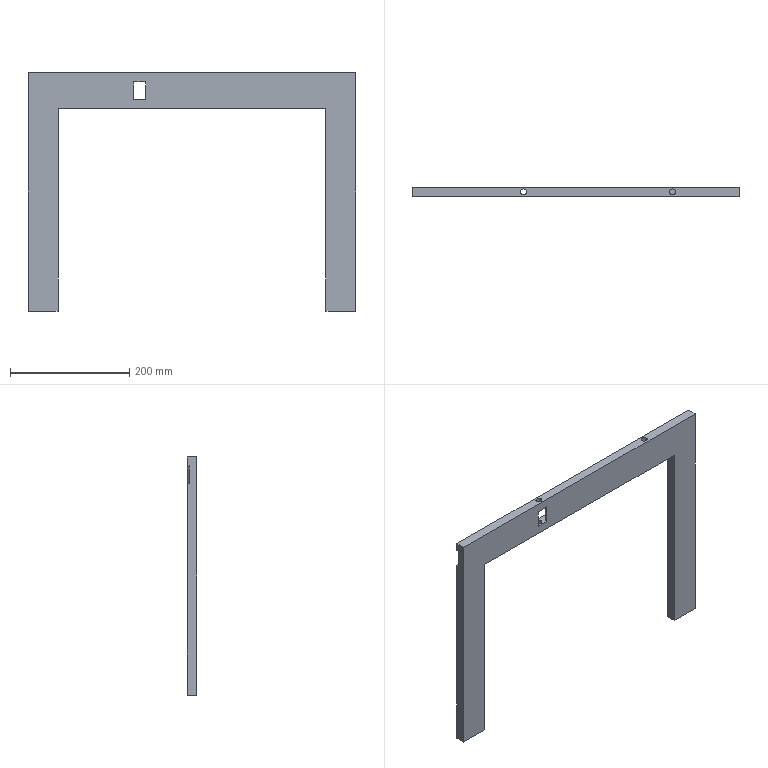Part | SolidWorks | features ICE 10, HoleWzd 3, Extrusion 1 | 1 solid | 25 faces | box 550 x 16 x 400 mm | volume 983083 mm3 | plane 19 | cylinder 6 | commonest cylinder face diameters 10 x6
STEP:
#1=CARTESIAN_POINT('',(182.,-8.,-60.));
#2=VERTEX_POINT('',#1);
#3=CARTESIAN_POINT('',(192.,-8.,-60.));
#4=VERTEX_POINT('',#3);
#5=CARTESIAN_POINT('',(187.,-8.,-60.));
#6=DIRECTION('',(0.,0.,1.));
#7=DIRECTION('',(1.,0.,0.));
#8=AXIS2_PLACEMENT_3D('',#5,#6,#7);
#9=CIRCLE('',#8,5.);
#10=EDGE_CURVE('',#2,#4,#9,.T.);
#11=ORIENTED_EDGE('',*,*,#10,.F.);
#12=CARTESIAN_POINT('',(182.,-8.,-45.));
#13=VERTEX_POINT('',#12);
#14=CARTESIAN_POINT('',(182.,-8.,-45.));
#15=DIRECTION('',(0.,0.,1.));
#16=VECTOR('',#15,1000.);
#17=LINE('',#14,#16);
#18=EDGE_CURVE('',#2,#13,#17,.T.);
#19=ORIENTED_EDGE('',*,*,#18,.T.);
#20=CARTESIAN_POINT('',(192.,-8.,-45.));
#21=VERTEX_POINT('',#20);
#22=CARTESIAN_POINT('',(187.,-8.,-45.));
#23=DIRECTION('',(0.,0.,1.));
#24=DIRECTION('',(1.,0.,0.));
#25=AXIS2_PLACEMENT_3D('',#22,#23,#24);
#26=CIRCLE('',#25,5.);
#27=EDGE_CURVE('',#13,#21,#26,.T.);
#28=ORIENTED_EDGE('',*,*,#27,.T.);
#29=CARTESIAN_POINT('',(192.,-8.,-45.));
#30=DIRECTION('',(0.,0.,1.));
#31=VECTOR('',#30,1000.);
#32=LINE('',#29,#31);
#33=EDGE_CURVE('',#4,#21,#32,.T.);
#34=ORIENTED_EDGE('',*,*,#33,.F.);
#35=EDGE_LOOP('',(#11,#19,#28,#34));
#36=FACE_OUTER_BOUND('',#35,.T.);
#37=CARTESIAN_POINT('',(187.,-8.,-45.));
#38=DIRECTION('',(0.,0.,1.));
#39=DIRECTION('',(1.,0.,0.));
#40=AXIS2_PLACEMENT_3D('',#37,#38,#39);
#41=CYLINDRICAL_SURFACE('',#40,5.);
#42=ADVANCED_FACE('',(#36),#41,.F.);
#43=CARTESIAN_POINT('',(192.,-8.,-15.));
#44=VERTEX_POINT('',#43);
#45=CARTESIAN_POINT('',(182.,-8.,-15.));
#46=VERTEX_POINT('',#45);
#47=CARTESIAN_POINT('',(187.,-8.,-15.));
#48=DIRECTION('',(0.,0.,-1.));
#49=DIRECTION('',(-1.,0.,0.));
#50=AXIS2_PLACEMENT_3D('',#47,#48,#49);
#51=CIRCLE('',#50,5.);
#52=EDGE_CURVE('',#44,#46,#51,.T.);
#53=ORIENTED_EDGE('',*,*,#52,.T.);
#54=CARTESIAN_POINT('',(182.,-8.,0.));
#55=VERTEX_POINT('',#54);
#56=CARTESIAN_POINT('',(182.,-8.,0.));
#57=DIRECTION('',(0.,0.,1.));
#58=VECTOR('',#57,1000.);
#59=LINE('',#56,#58);
#60=EDGE_CURVE('',#46,#55,#59,.T.);
#61=ORIENTED_EDGE('',*,*,#60,.T.);
#62=CARTESIAN_POINT('',(192.,-8.,0.));
#63=VERTEX_POINT('',#62);
#64=CARTESIAN_POINT('',(187.,-8.,0.));
#65=DIRECTION('',(0.,0.,1.));
#66=DIRECTION('',(1.,0.,0.));
#67=AXIS2_PLACEMENT_3D('',#64,#65,#66);
#68=CIRCLE('',#67,5.);
#69=EDGE_CURVE('',#55,#63,#68,.T.);
#70=ORIENTED_EDGE('',*,*,#69,.T.);
#71=CARTESIAN_POINT('',(192.,-8.,0.));
#72=DIRECTION('',(0.,0.,1.));
#73=VECTOR('',#72,1000.);
#74=LINE('',#71,#73);
#75=EDGE_CURVE('',#44,#63,#74,.T.);
#76=ORIENTED_EDGE('',*,*,#75,.F.);
#77=EDGE_LOOP('',(#53,#61,#70,#76));
#78=FACE_OUTER_BOUND('',#77,.T.);
#79=CARTESIAN_POINT('',(187.,-8.,0.));
#80=DIRECTION('',(0.,0.,1.));
#81=DIRECTION('',(1.,0.,0.));
#82=AXIS2_PLACEMENT_3D('',#79,#80,#81);
#83=CYLINDRICAL_SURFACE('',#82,5.);
#84=ADVANCED_FACE('',(#78),#83,.F.);
#85=CARTESIAN_POINT('',(432.,-8.,-20.));
#86=VERTEX_POINT('',#85);
#87=CARTESIAN_POINT('',(442.,-8.,-20.));
#88=VERTEX_POINT('',#87);
#89=CARTESIAN_POINT('',(437.,-8.,-20.));
#90=DIRECTION('',(0.,0.,1.));
#91=DIRECTION('',(1.,0.,0.));
#92=AXIS2_PLACEMENT_3D('',#89,#90,#91);
#93=CIRCLE('',#92,5.);
#94=EDGE_CURVE('',#86,#88,#93,.T.);
#95=ORIENTED_EDGE('',*,*,#94,.F.);
#96=CARTESIAN_POINT('',(432.,-8.,0.));
#97=VERTEX_POINT('',#96);
#98=CARTESIAN_POINT('',(432.,-8.,0.));
#99=DIRECTION('',(0.,0.,1.));
#100=VECTOR('',#99,1000.);
#101=LINE('',#98,#100);
#102=EDGE_CURVE('',#86,#97,#101,.T.);
#103=ORIENTED_EDGE('',*,*,#102,.T.);
#104=CARTESIAN_POINT('',(442.,-8.,0.));
#105=VERTEX_POINT('',#104);
#106=CARTESIAN_POINT('',(437.,-8.,0.));
#107=DIRECTION('',(0.,0.,1.));
#108=DIRECTION('',(1.,0.,0.));
#109=AXIS2_PLACEMENT_3D('',#106,#107,#108);
#110=CIRCLE('',#109,5.);
#111=EDGE_CURVE('',#97,#105,#110,.T.);
#112=ORIENTED_EDGE('',*,*,#111,.T.);
#113=CARTESIAN_POINT('',(442.,-8.,0.));
#114=DIRECTION('',(0.,0.,1.));
#115=VECTOR('',#114,1000.);
#116=LINE('',#113,#115);
#117=EDGE_CURVE('',#88,#105,#116,.T.);
#118=ORIENTED_EDGE('',*,*,#117,.F.);
#119=EDGE_LOOP('',(#95,#103,#112,#118));
#120=FACE_OUTER_BOUND('',#119,.T.);
#121=CARTESIAN_POINT('',(437.,-8.,0.));
#122=DIRECTION('',(0.,0.,1.));
#123=DIRECTION('',(1.,0.,0.));
#124=AXIS2_PLACEMENT_3D('',#121,#122,#123);
#125=CYLINDRICAL_SURFACE('',#124,5.);
#126=ADVANCED_FACE('',(#120),#125,.F.);
#127=CARTESIAN_POINT('',(437.,-8.,0.));
#128=DIRECTION('',(0.,0.,1.));
#129=DIRECTION('',(1.,0.,0.));
#130=AXIS2_PLACEMENT_3D('',#127,#128,#129);
#131=CIRCLE('',#130,5.);
#132=EDGE_CURVE('',#105,#97,#131,.T.);
#133=ORIENTED_EDGE('',*,*,#132,.F.);
#134=ORIENTED_EDGE('',*,*,#111,.F.);
#135=EDGE_LOOP('',(#133,#134));
#136=FACE_BOUND('',#135,.T.);
#137=CARTESIAN_POINT('',(0.,-16.,0.));
#138=VERTEX_POINT('',#137);
#139=CARTESIAN_POINT('',(550.,-16.,0.));
#140=VERTEX_POINT('',#139);
#141=CARTESIAN_POINT('',(355.,-16.,0.));
#142=DIRECTION('',(1.,0.,0.));
#143=VECTOR('',#142,1000.);
#144=LINE('',#141,#143);
#145=EDGE_CURVE('',#138,#140,#144,.T.);
#146=ORIENTED_EDGE('',*,*,#145,.T.);
#147=CARTESIAN_POINT('',(550.,0.,0.));
#148=VERTEX_POINT('',#147);
#149=CARTESIAN_POINT('',(550.,-16.,0.));
#150=DIRECTION('',(0.,-1.,0.));
#151=VECTOR('',#150,1000.);
#152=LINE('',#149,#151);
#153=EDGE_CURVE('',#148,#140,#152,.T.);
#154=ORIENTED_EDGE('',*,*,#153,.F.);
#155=CARTESIAN_POINT('',(0.,0.,0.));
#156=VERTEX_POINT('',#155);
#157=CARTESIAN_POINT('',(347.,0.,0.));
#158=DIRECTION('',(-1.,0.,0.));
#159=VECTOR('',#158,1000.);
#160=LINE('',#157,#159);
#161=EDGE_CURVE('',#148,#156,#160,.T.);
#162=ORIENTED_EDGE('',*,*,#161,.T.);
#163=CARTESIAN_POINT('',(0.,0.,0.));
#164=DIRECTION('',(0.,1.,0.));
#165=VECTOR('',#164,1000.);
#166=LINE('',#163,#165);
#167=EDGE_CURVE('',#138,#156,#166,.T.);
#168=ORIENTED_EDGE('',*,*,#167,.F.);
#169=EDGE_LOOP('',(#146,#154,#162,#168));
#170=FACE_OUTER_BOUND('',#169,.T.);
#171=CARTESIAN_POINT('',(187.,-8.,0.));
#172=DIRECTION('',(0.,0.,1.));
#173=DIRECTION('',(1.,0.,0.));
#174=AXIS2_PLACEMENT_3D('',#171,#172,#173);
#175=CIRCLE('',#174,5.);
#176=EDGE_CURVE('',#63,#55,#175,.T.);
#177=ORIENTED_EDGE('',*,*,#176,.F.);
#178=ORIENTED_EDGE('',*,*,#69,.F.);
#179=EDGE_LOOP('',(#177,#178));
#180=FACE_BOUND('',#179,.T.);
#181=CARTESIAN_POINT('',(0.,0.,0.));
#182=DIRECTION('',(0.,0.,-1.));
#183=DIRECTION('',(-1.,0.,0.));
#184=AXIS2_PLACEMENT_3D('',#181,#182,#183);
#185=PLANE('',#184);
#186=ADVANCED_FACE('',(#136,#170,#180),#185,.F.);
#187=CARTESIAN_POINT('',(550.,-16.,-400.));
#188=VERTEX_POINT('',#187);
#189=CARTESIAN_POINT('',(500.,-16.,-400.));
#190=VERTEX_POINT('',#189);
#191=CARTESIAN_POINT('',(0.,-16.,-400.));
#192=DIRECTION('',(-1.,0.,0.));
#193=VECTOR('',#192,1000.);
#194=LINE('',#191,#193);
#195=EDGE_CURVE('',#188,#190,#194,.T.);
#196=ORIENTED_EDGE('',*,*,#195,.T.);
#197=CARTESIAN_POINT('',(500.,0.,-400.));
#198=VERTEX_POINT('',#197);
#199=CARTESIAN_POINT('',(500.,-16.,-400.));
#200=DIRECTION('',(0.,1.,0.));
#201=VECTOR('',#200,1000.);
#202=LINE('',#199,#201);
#203=EDGE_CURVE('',#190,#198,#202,.T.);
#204=ORIENTED_EDGE('',*,*,#203,.T.);
#205=CARTESIAN_POINT('',(550.,0.,-400.));
#206=VERTEX_POINT('',#205);
#207=CARTESIAN_POINT('',(550.,0.,-400.));
#208=DIRECTION('',(1.,0.,0.));
#209=VECTOR('',#208,1000.);
#210=LINE('',#207,#209);
#211=EDGE_CURVE('',#198,#206,#210,.T.);
#212=ORIENTED_EDGE('',*,*,#211,.T.);
#213=CARTESIAN_POINT('',(550.,-16.,-400.));
#214=DIRECTION('',(0.,-1.,0.));
#215=VECTOR('',#214,1000.);
#216=LINE('',#213,#215);
#217=EDGE_CURVE('',#206,#188,#216,.T.);
#218=ORIENTED_EDGE('',*,*,#217,.T.);
#219=EDGE_LOOP('',(#196,#204,#212,#218));
#220=FACE_OUTER_BOUND('',#219,.T.);
#221=CARTESIAN_POINT('',(0.,0.,-400.));
#222=DIRECTION('',(0.,0.,1.));
#223=DIRECTION('',(1.,0.,0.));
#224=AXIS2_PLACEMENT_3D('',#221,#222,#223);
#225=PLANE('',#224);
#226=ADVANCED_FACE('',(#220),#225,.F.);
#227=CARTESIAN_POINT('',(197.,-13.,-45.));
#228=VERTEX_POINT('',#227);
#229=CARTESIAN_POINT('',(197.,-13.,-15.));
#230=VERTEX_POINT('',#229);
#231=CARTESIAN_POINT('',(197.,-13.,-45.));
#232=DIRECTION('',(0.,0.,1.));
#233=VECTOR('',#232,1000.);
#234=LINE('',#231,#233);
#235=EDGE_CURVE('',#228,#230,#234,.T.);
#236=ORIENTED_EDGE('',*,*,#235,.F.);
#237=CARTESIAN_POINT('',(197.,-16.,-45.));
#238=VERTEX_POINT('',#237);
#239=CARTESIAN_POINT('',(197.,-16.,-45.));
#240=DIRECTION('',(0.,1.,0.));
#241=VECTOR('',#240,1000.);
#242=LINE('',#239,#241);
#243=EDGE_CURVE('',#238,#228,#242,.T.);
#244=ORIENTED_EDGE('',*,*,#243,.F.);
#245=CARTESIAN_POINT('',(197.,-16.,-15.));
#246=VERTEX_POINT('',#245);
#247=CARTESIAN_POINT('',(197.,-16.,-15.));
#248=DIRECTION('',(0.,0.,-1.));
#249=VECTOR('',#248,1000.);
#250=LINE('',#247,#249);
#251=EDGE_CURVE('',#246,#238,#250,.T.);
#252=ORIENTED_EDGE('',*,*,#251,.F.);
#253=CARTESIAN_POINT('',(197.,-3.,-15.));
#254=DIRECTION('',(0.,-1.,0.));
#255=VECTOR('',#254,1000.);
#256=LINE('',#253,#255);
#257=EDGE_CURVE('',#230,#246,#256,.T.);
#258=ORIENTED_EDGE('',*,*,#257,.F.);
#259=EDGE_LOOP('',(#236,#244,#252,#258));
#260=FACE_OUTER_BOUND('',#259,.T.);
#261=CARTESIAN_POINT('',(197.,0.,0.));
#262=DIRECTION('',(1.,0.,0.));
#263=DIRECTION('',(0.,0.,-1.));
#264=AXIS2_PLACEMENT_3D('',#261,#262,#263);
#265=PLANE('',#264);
#266=ADVANCED_FACE('',(#260),#265,.F.);
#267=CARTESIAN_POINT('',(0.,-3.,-15.));
#268=VERTEX_POINT('',#267);
#269=CARTESIAN_POINT('',(177.,-3.,-15.));
#270=VERTEX_POINT('',#269);
#271=CARTESIAN_POINT('',(0.,-3.,-15.));
#272=DIRECTION('',(1.,0.,0.));
#273=VECTOR('',#272,1000.);
#274=LINE('',#271,#273);
#275=EDGE_CURVE('',#268,#270,#274,.T.);
#276=ORIENTED_EDGE('',*,*,#275,.T.);
#277=CARTESIAN_POINT('',(177.,-3.,-45.));
#278=VERTEX_POINT('',#277);
#279=CARTESIAN_POINT('',(177.,-3.,-45.));
#280=DIRECTION('',(0.,0.,1.));
#281=VECTOR('',#280,1000.);
#282=LINE('',#279,#281);
#283=EDGE_CURVE('',#278,#270,#282,.T.);
#284=ORIENTED_EDGE('',*,*,#283,.F.);
#285=CARTESIAN_POINT('',(0.,-3.,-45.));
#286=VERTEX_POINT('',#285);
#287=CARTESIAN_POINT('',(347.,-3.,-45.));
#288=DIRECTION('',(-1.,0.,0.));
#289=VECTOR('',#288,1000.);
#290=LINE('',#287,#289);
#291=EDGE_CURVE('',#278,#286,#290,.T.);
#292=ORIENTED_EDGE('',*,*,#291,.T.);
#293=CARTESIAN_POINT('',(0.,-3.,-45.));
#294=DIRECTION('',(0.,0.,1.));
#295=VECTOR('',#294,1000.);
#296=LINE('',#293,#295);
#297=EDGE_CURVE('',#286,#268,#296,.T.);
#298=ORIENTED_EDGE('',*,*,#297,.T.);
#299=EDGE_LOOP('',(#276,#284,#292,#298));
#300=FACE_OUTER_BOUND('',#299,.T.);
#301=CARTESIAN_POINT('',(0.,-3.,0.));
#302=DIRECTION('',(0.,1.,0.));
#303=DIRECTION('',(0.,0.,1.));
#304=AXIS2_PLACEMENT_3D('',#301,#302,#303);
#305=PLANE('',#304);
#306=ADVANCED_FACE('',(#300),#305,.T.);
#307=CARTESIAN_POINT('',(177.,-16.,-45.));
#308=VERTEX_POINT('',#307);
#309=CARTESIAN_POINT('',(0.,-16.,-45.));
#310=DIRECTION('',(-1.,0.,0.));
#311=VECTOR('',#310,1000.);
#312=LINE('',#309,#311);
#313=EDGE_CURVE('',#238,#308,#312,.T.);
#314=ORIENTED_EDGE('',*,*,#313,.T.);
#315=CARTESIAN_POINT('',(177.,-16.,-15.));
#316=VERTEX_POINT('',#315);
#317=CARTESIAN_POINT('',(177.,-16.,-15.));
#318=DIRECTION('',(0.,0.,-1.));
#319=VECTOR('',#318,1000.);
#320=LINE('',#317,#319);
#321=EDGE_CURVE('',#316,#308,#320,.T.);
#322=ORIENTED_EDGE('',*,*,#321,.F.);
#323=CARTESIAN_POINT('',(177.,-16.,-15.));
#324=DIRECTION('',(1.,0.,0.));
#325=VECTOR('',#324,1000.);
#326=LINE('',#323,#325);
#327=EDGE_CURVE('',#316,#246,#326,.T.);
#328=ORIENTED_EDGE('',*,*,#327,.T.);
#329=ORIENTED_EDGE('',*,*,#251,.T.);
#330=EDGE_LOOP('',(#314,#322,#328,#329));
#331=FACE_BOUND('',#330,.T.);
#332=CARTESIAN_POINT('',(50.,-16.,-60.));
#333=VERTEX_POINT('',#332);
#334=CARTESIAN_POINT('',(500.,-16.,-60.));
#335=VERTEX_POINT('',#334);
#336=CARTESIAN_POINT('',(50.,-16.,-60.));
#337=DIRECTION('',(1.,0.,0.));
#338=VECTOR('',#337,1000.);
#339=LINE('',#336,#338);
#340=EDGE_CURVE('',#333,#335,#339,.T.);
#341=ORIENTED_EDGE('',*,*,#340,.T.);
#342=CARTESIAN_POINT('',(500.,-16.,-60.));
#343=DIRECTION('',(0.,0.,-1.));
#344=VECTOR('',#343,1000.);
#345=LINE('',#342,#344);
#346=EDGE_CURVE('',#335,#190,#345,.T.);
#347=ORIENTED_EDGE('',*,*,#346,.T.);
#348=ORIENTED_EDGE('',*,*,#195,.F.);
#349=CARTESIAN_POINT('',(550.,-16.,-45.));
#350=DIRECTION('',(0.,0.,-1.));
#351=VECTOR('',#350,1000.);
#352=LINE('',#349,#351);
#353=EDGE_CURVE('',#140,#188,#352,.T.);
#354=ORIENTED_EDGE('',*,*,#353,.F.);
#355=ORIENTED_EDGE('',*,*,#145,.F.);
#356=CARTESIAN_POINT('',(0.,-16.,-400.));
#357=VERTEX_POINT('',#356);
#358=CARTESIAN_POINT('',(0.,-16.,0.));
#359=DIRECTION('',(0.,0.,1.));
#360=VECTOR('',#359,1000.);
#361=LINE('',#358,#360);
#362=EDGE_CURVE('',#357,#138,#361,.T.);
#363=ORIENTED_EDGE('',*,*,#362,.F.);
#364=CARTESIAN_POINT('',(50.,-16.,-400.));
#365=VERTEX_POINT('',#364);
#366=CARTESIAN_POINT('',(0.,-16.,-400.));
#367=DIRECTION('',(-1.,0.,0.));
#368=VECTOR('',#367,1000.);
#369=LINE('',#366,#368);
#370=EDGE_CURVE('',#365,#357,#369,.T.);
#371=ORIENTED_EDGE('',*,*,#370,.F.);
#372=CARTESIAN_POINT('',(50.,-16.,-400.));
#373=DIRECTION('',(0.,0.,1.));
#374=VECTOR('',#373,1000.);
#375=LINE('',#372,#374);
#376=EDGE_CURVE('',#365,#333,#375,.T.);
#377=ORIENTED_EDGE('',*,*,#376,.T.);
#378=EDGE_LOOP('',(#341,#347,#348,#354,#355,#363,#371,#377));
#379=FACE_OUTER_BOUND('',#378,.T.);
#380=CARTESIAN_POINT('',(0.,-16.,0.));
#381=DIRECTION('',(0.,1.,0.));
#382=DIRECTION('',(0.,0.,1.));
#383=AXIS2_PLACEMENT_3D('',#380,#381,#382);
#384=PLANE('',#383);
#385=ADVANCED_FACE('',(#331,#379),#384,.F.);
#386=CARTESIAN_POINT('',(347.,-8.,-45.));
#387=VERTEX_POINT('',#386);
#388=CARTESIAN_POINT('',(355.,0.,-45.));
#389=VERTEX_POINT('',#388);
#390=CARTESIAN_POINT('',(347.,-8.,-45.));
#391=DIRECTION('',(0.7071,0.7071,0.));
#392=VECTOR('',#391,1000.);
#393=LINE('',#390,#392);
#394=EDGE_CURVE('',#387,#389,#393,.T.);
#395=ORIENTED_EDGE('',*,*,#394,.F.);
#396=CARTESIAN_POINT('',(347.,-8.,-15.));
#397=VERTEX_POINT('',#396);
#398=CARTESIAN_POINT('',(347.,-8.,-15.));
#399=DIRECTION('',(0.,0.,-1.));
#400=VECTOR('',#399,1000.);
#401=LINE('',#398,#400);
#402=EDGE_CURVE('',#397,#387,#401,.T.);
#403=ORIENTED_EDGE('',*,*,#402,.F.);
#404=CARTESIAN_POINT('',(355.,0.,-15.));
#405=VERTEX_POINT('',#404);
#406=CARTESIAN_POINT('',(347.,-8.,-15.));
#407=DIRECTION('',(0.7071,0.7071,0.));
#408=VECTOR('',#407,1000.);
#409=LINE('',#406,#408);
#410=EDGE_CURVE('',#397,#405,#409,.T.);
#411=ORIENTED_EDGE('',*,*,#410,.T.);
#412=CARTESIAN_POINT('',(355.,0.,-15.));
#413=DIRECTION('',(0.,0.,-1.));
#414=VECTOR('',#413,1000.);
#415=LINE('',#412,#414);
#416=EDGE_CURVE('',#405,#389,#415,.T.);
#417=ORIENTED_EDGE('',*,*,#416,.T.);
#418=EDGE_LOOP('',(#395,#403,#411,#417));
#419=FACE_OUTER_BOUND('',#418,.T.);
#420=CARTESIAN_POINT('',(347.,-8.,-15.));
#421=DIRECTION('',(-0.7071,0.7071,0.));
#422=DIRECTION('',(-0.7071,-0.7071,0.));
#423=AXIS2_PLACEMENT_3D('',#420,#421,#422);
#424=PLANE('',#423);
#425=ADVANCED_FACE('',(#419),#424,.T.);
#426=ORIENTED_EDGE('',*,*,#52,.F.);
#427=CARTESIAN_POINT('',(187.,-8.,-15.));
#428=DIRECTION('',(0.,0.,-1.));
#429=DIRECTION('',(-1.,0.,0.));
#430=AXIS2_PLACEMENT_3D('',#427,#428,#429);
#431=CIRCLE('',#430,5.);
#432=EDGE_CURVE('',#46,#44,#431,.T.);
#433=ORIENTED_EDGE('',*,*,#432,.F.);
#434=EDGE_LOOP('',(#426,#433));
#435=FACE_BOUND('',#434,.T.);
#436=ORIENTED_EDGE('',*,*,#410,.F.);
#437=CARTESIAN_POINT('',(347.,-13.,-15.));
#438=VERTEX_POINT('',#437);
#439=CARTESIAN_POINT('',(347.,-13.,-15.));
#440=DIRECTION('',(0.,1.,0.));
#441=VECTOR('',#440,1000.);
#442=LINE('',#439,#441);
#443=EDGE_CURVE('',#438,#397,#442,.T.);
#444=ORIENTED_EDGE('',*,*,#443,.F.);
#445=CARTESIAN_POINT('',(197.,-13.,-15.));
#446=DIRECTION('',(1.,0.,0.));
#447=VECTOR('',#446,1000.);
#448=LINE('',#445,#447);
#449=EDGE_CURVE('',#230,#438,#448,.T.);
#450=ORIENTED_EDGE('',*,*,#449,.F.);
#451=ORIENTED_EDGE('',*,*,#257,.T.);
#452=ORIENTED_EDGE('',*,*,#327,.F.);
#453=CARTESIAN_POINT('',(177.,-3.,-15.));
#454=DIRECTION('',(0.,-1.,0.));
#455=VECTOR('',#454,1000.);
#456=LINE('',#453,#455);
#457=EDGE_CURVE('',#270,#316,#456,.T.);
#458=ORIENTED_EDGE('',*,*,#457,.F.);
#459=ORIENTED_EDGE('',*,*,#275,.F.);
#460=CARTESIAN_POINT('',(0.,0.,-15.));
#461=VERTEX_POINT('',#460);
#462=CARTESIAN_POINT('',(0.,-3.,-15.));
#463=DIRECTION('',(0.,1.,0.));
#464=VECTOR('',#463,1000.);
#465=LINE('',#462,#464);
#466=EDGE_CURVE('',#268,#461,#465,.T.);
#467=ORIENTED_EDGE('',*,*,#466,.T.);
#468=CARTESIAN_POINT('',(347.,0.,-15.));
#469=DIRECTION('',(-1.,0.,0.));
#470=VECTOR('',#469,1000.);
#471=LINE('',#468,#470);
#472=EDGE_CURVE('',#405,#461,#471,.T.);
#473=ORIENTED_EDGE('',*,*,#472,.F.);
#474=EDGE_LOOP('',(#436,#444,#450,#451,#452,#458,#459,#467,#473));
#475=FACE_OUTER_BOUND('',#474,.T.);
#476=CARTESIAN_POINT('',(0.,0.,-15.));
#477=DIRECTION('',(0.,0.,-1.));
#478=DIRECTION('',(-1.,0.,0.));
#479=AXIS2_PLACEMENT_3D('',#476,#477,#478);
#480=PLANE('',#479);
#481=ADVANCED_FACE('',(#435,#475),#480,.T.);
#482=ORIENTED_EDGE('',*,*,#211,.F.);
#483=CARTESIAN_POINT('',(500.,0.,-60.));
#484=VERTEX_POINT('',#483);
#485=CARTESIAN_POINT('',(500.,0.,-60.));
#486=DIRECTION('',(0.,0.,-1.));
#487=VECTOR('',#486,1000.);
#488=LINE('',#485,#487);
#489=EDGE_CURVE('',#484,#198,#488,.T.);
#490=ORIENTED_EDGE('',*,*,#489,.F.);
#491=CARTESIAN_POINT('',(50.,0.,-60.));
#492=VERTEX_POINT('',#491);
#493=CARTESIAN_POINT('',(50.,0.,-60.));
#494=DIRECTION('',(1.,0.,0.));
#495=VECTOR('',#494,1000.);
#496=LINE('',#493,#495);
#497=EDGE_CURVE('',#492,#484,#496,.T.);
#498=ORIENTED_EDGE('',*,*,#497,.F.);
#499=CARTESIAN_POINT('',(50.,0.,-400.));
#500=VERTEX_POINT('',#499);
#501=CARTESIAN_POINT('',(50.,0.,-400.));
#502=DIRECTION('',(0.,0.,1.));
#503=VECTOR('',#502,1000.);
#504=LINE('',#501,#503);
#505=EDGE_CURVE('',#500,#492,#504,.T.);
#506=ORIENTED_EDGE('',*,*,#505,.F.);
#507=CARTESIAN_POINT('',(0.,0.,-400.));
#508=VERTEX_POINT('',#507);
#509=CARTESIAN_POINT('',(550.,0.,-400.));
#510=DIRECTION('',(1.,0.,0.));
#511=VECTOR('',#510,1000.);
#512=LINE('',#509,#511);
#513=EDGE_CURVE('',#508,#500,#512,.T.);
#514=ORIENTED_EDGE('',*,*,#513,.F.);
#515=CARTESIAN_POINT('',(0.,0.,-45.));
#516=VERTEX_POINT('',#515);
#517=CARTESIAN_POINT('',(0.,0.,-400.));
#518=DIRECTION('',(0.,0.,1.));
#519=VECTOR('',#518,1000.);
#520=LINE('',#517,#519);
#521=EDGE_CURVE('',#508,#516,#520,.T.);
#522=ORIENTED_EDGE('',*,*,#521,.T.);
#523=CARTESIAN_POINT('',(550.,0.,-45.));
#524=DIRECTION('',(1.,0.,0.));
#525=VECTOR('',#524,1000.);
#526=LINE('',#523,#525);
#527=EDGE_CURVE('',#516,#389,#526,.T.);
#528=ORIENTED_EDGE('',*,*,#527,.T.);
#529=ORIENTED_EDGE('',*,*,#416,.F.);
#530=ORIENTED_EDGE('',*,*,#472,.T.);
#531=CARTESIAN_POINT('',(0.,0.,-45.));
#532=DIRECTION('',(0.,0.,-1.));
#533=VECTOR('',#532,1000.);
#534=LINE('',#531,#533);
#535=EDGE_CURVE('',#156,#461,#534,.T.);
#536=ORIENTED_EDGE('',*,*,#535,.F.);
#537=ORIENTED_EDGE('',*,*,#161,.F.);
#538=CARTESIAN_POINT('',(550.,0.,0.));
#539=DIRECTION('',(0.,0.,1.));
#540=VECTOR('',#539,1000.);
#541=LINE('',#538,#540);
#542=EDGE_CURVE('',#206,#148,#541,.T.);
#543=ORIENTED_EDGE('',*,*,#542,.F.);
#544=EDGE_LOOP('',(#482,#490,#498,#506,#514,#522,#528,#529,#530,#536,#537,#543));
#545=FACE_OUTER_BOUND('',#544,.T.);
#546=CARTESIAN_POINT('',(347.,0.,0.));
#547=DIRECTION('',(0.,-1.,0.));
#548=DIRECTION('',(0.,0.,-1.));
#549=AXIS2_PLACEMENT_3D('',#546,#547,#548);
#550=PLANE('',#549);
#551=ADVANCED_FACE('',(#545),#550,.F.);
#552=ORIENTED_EDGE('',*,*,#542,.T.);
#553=ORIENTED_EDGE('',*,*,#153,.T.);
#554=ORIENTED_EDGE('',*,*,#353,.T.);
#555=ORIENTED_EDGE('',*,*,#217,.F.);
#556=EDGE_LOOP('',(#552,#553,#554,#555));
#557=FACE_OUTER_BOUND('',#556,.T.);
#558=CARTESIAN_POINT('',(550.,0.,0.));
#559=DIRECTION('',(-1.,0.,0.));
#560=DIRECTION('',(0.,0.,1.));
#561=AXIS2_PLACEMENT_3D('',#558,#559,#560);
#562=PLANE('',#561);
#563=ADVANCED_FACE('',(#557),#562,.F.);
#564=ORIENTED_EDGE('',*,*,#535,.T.);
#565=ORIENTED_EDGE('',*,*,#466,.F.);
#566=ORIENTED_EDGE('',*,*,#297,.F.);
#567=CARTESIAN_POINT('',(0.,0.,-45.));
#568=DIRECTION('',(0.,1.,0.));
#569=VECTOR('',#568,1000.);
#570=LINE('',#567,#569);
#571=EDGE_CURVE('',#286,#516,#570,.T.);
#572=ORIENTED_EDGE('',*,*,#571,.T.);
#573=ORIENTED_EDGE('',*,*,#521,.F.);
#574=CARTESIAN_POINT('',(0.,0.,-400.));
#575=DIRECTION('',(0.,1.,0.));
#576=VECTOR('',#575,1000.);
#577=LINE('',#574,#576);
#578=EDGE_CURVE('',#357,#508,#577,.T.);
#579=ORIENTED_EDGE('',*,*,#578,.F.);
#580=ORIENTED_EDGE('',*,*,#362,.T.);
#581=ORIENTED_EDGE('',*,*,#167,.T.);
#582=EDGE_LOOP('',(#564,#565,#566,#572,#573,#579,#580,#581));
#583=FACE_OUTER_BOUND('',#582,.T.);
#584=CARTESIAN_POINT('',(0.,0.,0.));
#585=DIRECTION('',(1.,0.,0.));
#586=DIRECTION('',(0.,0.,-1.));
#587=AXIS2_PLACEMENT_3D('',#584,#585,#586);
#588=PLANE('',#587);
#589=ADVANCED_FACE('',(#583),#588,.F.);
#590=ORIENTED_EDGE('',*,*,#457,.T.);
#591=ORIENTED_EDGE('',*,*,#321,.T.);
#592=CARTESIAN_POINT('',(177.,-16.,-45.));
#593=DIRECTION('',(0.,1.,0.));
#594=VECTOR('',#593,1000.);
#595=LINE('',#592,#594);
#596=EDGE_CURVE('',#308,#278,#595,.T.);
#597=ORIENTED_EDGE('',*,*,#596,.T.);
#598=ORIENTED_EDGE('',*,*,#283,.T.);
#599=EDGE_LOOP('',(#590,#591,#597,#598));
#600=FACE_OUTER_BOUND('',#599,.T.);
#601=CARTESIAN_POINT('',(177.,0.,0.));
#602=DIRECTION('',(1.,0.,0.));
#603=DIRECTION('',(0.,0.,-1.));
#604=AXIS2_PLACEMENT_3D('',#601,#602,#603);
#605=PLANE('',#604);
#606=ADVANCED_FACE('',(#600),#605,.T.);
#607=ORIENTED_EDGE('',*,*,#402,.T.);
#608=CARTESIAN_POINT('',(347.,-13.,-45.));
#609=VERTEX_POINT('',#608);
#610=CARTESIAN_POINT('',(347.,-13.,-45.));
#611=DIRECTION('',(0.,1.,0.));
#612=VECTOR('',#611,1000.);
#613=LINE('',#610,#612);
#614=EDGE_CURVE('',#609,#387,#613,.T.);
#615=ORIENTED_EDGE('',*,*,#614,.F.);
#616=CARTESIAN_POINT('',(347.,-13.,-15.));
#617=DIRECTION('',(0.,0.,-1.));
#618=VECTOR('',#617,1000.);
#619=LINE('',#616,#618);
#620=EDGE_CURVE('',#438,#609,#619,.T.);
#621=ORIENTED_EDGE('',*,*,#620,.F.);
#622=ORIENTED_EDGE('',*,*,#443,.T.);
#623=EDGE_LOOP('',(#607,#615,#621,#622));
#624=FACE_OUTER_BOUND('',#623,.T.);
#625=CARTESIAN_POINT('',(347.,-13.,-15.));
#626=DIRECTION('',(1.,0.,0.));
#627=DIRECTION('',(0.,0.,-1.));
#628=AXIS2_PLACEMENT_3D('',#625,#626,#627);
#629=PLANE('',#628);
#630=ADVANCED_FACE('',(#624),#629,.F.);
#631=ORIENTED_EDGE('',*,*,#449,.T.);
#632=ORIENTED_EDGE('',*,*,#620,.T.);
#633=CARTESIAN_POINT('',(347.,-13.,-45.));
#634=DIRECTION('',(-1.,0.,0.));
#635=VECTOR('',#634,1000.);
#636=LINE('',#633,#635);
#637=EDGE_CURVE('',#609,#228,#636,.T.);
#638=ORIENTED_EDGE('',*,*,#637,.T.);
#639=ORIENTED_EDGE('',*,*,#235,.T.);
#640=EDGE_LOOP('',(#631,#632,#638,#639));
#641=FACE_OUTER_BOUND('',#640,.T.);
#642=CARTESIAN_POINT('',(0.,-13.,0.));
#643=DIRECTION('',(0.,1.,0.));
#644=DIRECTION('',(0.,0.,1.));
#645=AXIS2_PLACEMENT_3D('',#642,#643,#644);
#646=PLANE('',#645);
#647=ADVANCED_FACE('',(#641),#646,.T.);
#648=CARTESIAN_POINT('',(187.,-8.,-45.));
#649=DIRECTION('',(0.,0.,1.));
#650=DIRECTION('',(1.,0.,0.));
#651=AXIS2_PLACEMENT_3D('',#648,#649,#650);
#652=CIRCLE('',#651,5.);
#653=EDGE_CURVE('',#21,#13,#652,.T.);
#654=ORIENTED_EDGE('',*,*,#653,.F.);
#655=ORIENTED_EDGE('',*,*,#27,.F.);
#656=EDGE_LOOP('',(#654,#655));
#657=FACE_BOUND('',#656,.T.);
#658=ORIENTED_EDGE('',*,*,#571,.F.);
#659=ORIENTED_EDGE('',*,*,#291,.F.);
#660=ORIENTED_EDGE('',*,*,#596,.F.);
#661=ORIENTED_EDGE('',*,*,#313,.F.);
#662=ORIENTED_EDGE('',*,*,#243,.T.);
#663=ORIENTED_EDGE('',*,*,#637,.F.);
#664=ORIENTED_EDGE('',*,*,#614,.T.);
#665=ORIENTED_EDGE('',*,*,#394,.T.);
#666=ORIENTED_EDGE('',*,*,#527,.F.);
#667=EDGE_LOOP('',(#658,#659,#660,#661,#662,#663,#664,#665,#666));
#668=FACE_OUTER_BOUND('',#667,.T.);
#669=CARTESIAN_POINT('',(0.,0.,-45.));
#670=DIRECTION('',(0.,0.,1.));
#671=DIRECTION('',(1.,0.,0.));
#672=AXIS2_PLACEMENT_3D('',#669,#670,#671);
#673=PLANE('',#672);
#674=ADVANCED_FACE('',(#657,#668),#673,.T.);
#675=ORIENTED_EDGE('',*,*,#513,.T.);
#676=CARTESIAN_POINT('',(50.,-16.,-400.));
#677=DIRECTION('',(0.,1.,0.));
#678=VECTOR('',#677,1000.);
#679=LINE('',#676,#678);
#680=EDGE_CURVE('',#365,#500,#679,.T.);
#681=ORIENTED_EDGE('',*,*,#680,.F.);
#682=ORIENTED_EDGE('',*,*,#370,.T.);
#683=ORIENTED_EDGE('',*,*,#578,.T.);
#684=EDGE_LOOP('',(#675,#681,#682,#683));
#685=FACE_OUTER_BOUND('',#684,.T.);
#686=CARTESIAN_POINT('',(0.,0.,-400.));
#687=DIRECTION('',(0.,0.,1.));
#688=DIRECTION('',(1.,0.,0.));
#689=AXIS2_PLACEMENT_3D('',#686,#687,#688);
#690=PLANE('',#689);
#691=ADVANCED_FACE('',(#685),#690,.F.);
#692=ORIENTED_EDGE('',*,*,#489,.T.);
#693=ORIENTED_EDGE('',*,*,#203,.F.);
#694=ORIENTED_EDGE('',*,*,#346,.F.);
#695=CARTESIAN_POINT('',(500.,-16.,-60.));
#696=DIRECTION('',(0.,1.,0.));
#697=VECTOR('',#696,1000.);
#698=LINE('',#695,#697);
#699=EDGE_CURVE('',#335,#484,#698,.T.);
#700=ORIENTED_EDGE('',*,*,#699,.T.);
#701=EDGE_LOOP('',(#692,#693,#694,#700));
#702=FACE_OUTER_BOUND('',#701,.T.);
#703=CARTESIAN_POINT('',(500.,-16.,-60.));
#704=DIRECTION('',(1.,0.,0.));
#705=DIRECTION('',(0.,0.,-1.));
#706=AXIS2_PLACEMENT_3D('',#703,#704,#705);
#707=PLANE('',#706);
#708=ADVANCED_FACE('',(#702),#707,.F.);
#709=CARTESIAN_POINT('',(187.,-8.,-60.));
#710=DIRECTION('',(0.,0.,1.));
#711=DIRECTION('',(1.,0.,0.));
#712=AXIS2_PLACEMENT_3D('',#709,#710,#711);
#713=CIRCLE('',#712,5.);
#714=EDGE_CURVE('',#4,#2,#713,.T.);
#715=ORIENTED_EDGE('',*,*,#714,.T.);
#716=ORIENTED_EDGE('',*,*,#10,.T.);
#717=EDGE_LOOP('',(#715,#716));
#718=FACE_BOUND('',#717,.T.);
#719=ORIENTED_EDGE('',*,*,#497,.T.);
#720=ORIENTED_EDGE('',*,*,#699,.F.);
#721=ORIENTED_EDGE('',*,*,#340,.F.);
#722=CARTESIAN_POINT('',(50.,-16.,-60.));
#723=DIRECTION('',(0.,1.,0.));
#724=VECTOR('',#723,1000.);
#725=LINE('',#722,#724);
#726=EDGE_CURVE('',#333,#492,#725,.T.);
#727=ORIENTED_EDGE('',*,*,#726,.T.);
#728=EDGE_LOOP('',(#719,#720,#721,#727));
#729=FACE_OUTER_BOUND('',#728,.T.);
#730=CARTESIAN_POINT('',(50.,-16.,-60.));
#731=DIRECTION('',(0.,0.,1.));
#732=DIRECTION('',(1.,0.,0.));
#733=AXIS2_PLACEMENT_3D('',#730,#731,#732);
#734=PLANE('',#733);
#735=ADVANCED_FACE('',(#718,#729),#734,.F.);
#736=ORIENTED_EDGE('',*,*,#505,.T.);
#737=ORIENTED_EDGE('',*,*,#726,.F.);
#738=ORIENTED_EDGE('',*,*,#376,.F.);
#739=ORIENTED_EDGE('',*,*,#680,.T.);
#740=EDGE_LOOP('',(#736,#737,#738,#739));
#741=FACE_OUTER_BOUND('',#740,.T.);
#742=CARTESIAN_POINT('',(50.,-16.,-400.));
#743=DIRECTION('',(-1.,0.,0.));
#744=DIRECTION('',(0.,0.,1.));
#745=AXIS2_PLACEMENT_3D('',#742,#743,#744);
#746=PLANE('',#745);
#747=ADVANCED_FACE('',(#741),#746,.F.);
#748=CARTESIAN_POINT('',(437.,-8.,-20.));
#749=DIRECTION('',(0.,0.,1.));
#750=DIRECTION('',(1.,0.,0.));
#751=AXIS2_PLACEMENT_3D('',#748,#749,#750);
#752=CIRCLE('',#751,5.);
#753=EDGE_CURVE('',#88,#86,#752,.T.);
#754=ORIENTED_EDGE('',*,*,#753,.T.);
#755=ORIENTED_EDGE('',*,*,#94,.T.);
#756=EDGE_LOOP('',(#754,#755));
#757=FACE_OUTER_BOUND('',#756,.T.);
#758=CARTESIAN_POINT('',(437.,-8.,-20.));
#759=DIRECTION('',(0.,0.,-1.));
#760=DIRECTION('',(-1.,0.,0.));
#761=AXIS2_PLACEMENT_3D('',#758,#759,#760);
#762=PLANE('',#761);
#763=ADVANCED_FACE('',(#757),#762,.F.);
#764=ORIENTED_EDGE('',*,*,#102,.F.);
#765=ORIENTED_EDGE('',*,*,#753,.F.);
#766=ORIENTED_EDGE('',*,*,#117,.T.);
#767=ORIENTED_EDGE('',*,*,#132,.T.);
#768=EDGE_LOOP('',(#764,#765,#766,#767));
#769=FACE_OUTER_BOUND('',#768,.T.);
#770=CARTESIAN_POINT('',(437.,-8.,0.));
#771=DIRECTION('',(0.,0.,1.));
#772=DIRECTION('',(1.,0.,0.));
#773=AXIS2_PLACEMENT_3D('',#770,#771,#772);
#774=CYLINDRICAL_SURFACE('',#773,5.);
#775=ADVANCED_FACE('',(#769),#774,.F.);
#776=ORIENTED_EDGE('',*,*,#60,.F.);
#777=ORIENTED_EDGE('',*,*,#432,.T.);
#778=ORIENTED_EDGE('',*,*,#75,.T.);
#779=ORIENTED_EDGE('',*,*,#176,.T.);
#780=EDGE_LOOP('',(#776,#777,#778,#779));
#781=FACE_OUTER_BOUND('',#780,.T.);
#782=CARTESIAN_POINT('',(187.,-8.,0.));
#783=DIRECTION('',(0.,0.,1.));
#784=DIRECTION('',(1.,0.,0.));
#785=AXIS2_PLACEMENT_3D('',#782,#783,#784);
#786=CYLINDRICAL_SURFACE('',#785,5.);
#787=ADVANCED_FACE('',(#781),#786,.F.);
#788=ORIENTED_EDGE('',*,*,#18,.F.);
#789=ORIENTED_EDGE('',*,*,#714,.F.);
#790=ORIENTED_EDGE('',*,*,#33,.T.);
#791=ORIENTED_EDGE('',*,*,#653,.T.);
#792=EDGE_LOOP('',(#788,#789,#790,#791));
#793=FACE_OUTER_BOUND('',#792,.T.);
#794=CARTESIAN_POINT('',(187.,-8.,-45.));
#795=DIRECTION('',(0.,0.,1.));
#796=DIRECTION('',(1.,0.,0.));
#797=AXIS2_PLACEMENT_3D('',#794,#795,#796);
#798=CYLINDRICAL_SURFACE('',#797,5.);
#799=ADVANCED_FACE('',(#793),#798,.F.);
#800=CLOSED_SHELL('',(#42,#84,#126,#186,#226,#266,#306,#385,#425,#481,#551,#563,#589,#606,#630,#647,#674,#691,#708,#735,#747,#763,#775,#787,#799));
#801=MANIFOLD_SOLID_BREP('',#800);
#802=CARTESIAN_POINT('',(0.,0.,0.));
#803=DIRECTION('',(0.,0.,1.));
#804=DIRECTION('',(1.,0.,0.));
#805=AXIS2_PLACEMENT_3D('',#802,#803,#804);
#806=(LENGTH_UNIT()NAMED_UNIT(*)SI_UNIT(.MILLI.,.METRE.));
#807=UNCERTAINTY_MEASURE_WITH_UNIT(LENGTH_MEASURE(0.00001),#806,'','');
#808=(NAMED_UNIT(*)PLANE_ANGLE_UNIT()SI_UNIT($,.RADIAN.));
#809=(NAMED_UNIT(*)SI_UNIT($,.STERADIAN.)SOLID_ANGLE_UNIT());
#810=(GEOMETRIC_REPRESENTATION_CONTEXT(3)GLOBAL_UNCERTAINTY_ASSIGNED_CONTEXT((#807))GLOBAL_UNIT_ASSIGNED_CONTEXT((#806,#808,#809))REPRESENTATION_CONTEXT('',''));
#811=ADVANCED_BREP_SHAPE_REPRESENTATION('',(#801,#805),#810);